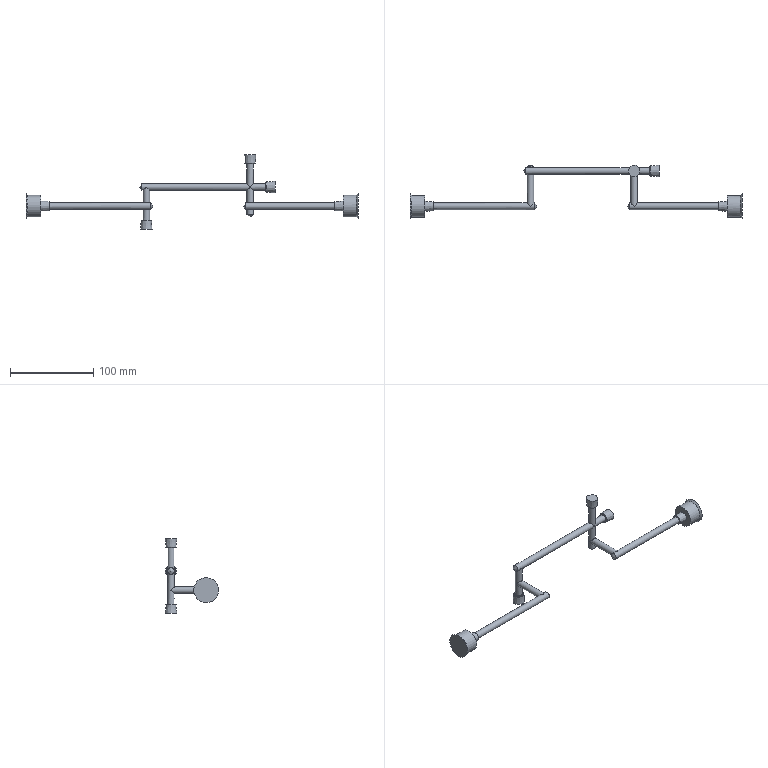Part | STEP file | COOLING-COR_id198_x_t | 1 solid | 37 faces | box 400 x 64.384 x 90 mm | volume 53366 mm3 | cone 14 | plane 12 | cylinder 11 | commonest cylinder face diameters 8 x9 26 x2
STEP:
#1=CARTESIAN_POINT('',(-200.,-80.5,0.));
#2=VERTEX_POINT('',#1);
#3=CARTESIAN_POINT('',(-200.,-80.5,-15.));
#4=DIRECTION('',(1.,0.,0.));
#5=DIRECTION('',(0.,0.,1.));
#6=AXIS2_PLACEMENT_3D('',#3,#4,#5);
#7=CIRCLE('',#6,15.);
#8=EDGE_CURVE('',#2,#2,#7,.T.);
#9=ORIENTED_EDGE('',*,*,#8,.F.);
#10=EDGE_LOOP('',(#9));
#11=FACE_OUTER_BOUND('',#10,.T.);
#12=CARTESIAN_POINT('',(-200.,-80.5,-15.));
#13=DIRECTION('',(1.,0.,0.));
#14=DIRECTION('',(0.,0.,-1.));
#15=AXIS2_PLACEMENT_3D('',#12,#13,#14);
#16=PLANE('',#15);
#17=ADVANCED_FACE('',(#11),#16,.F.);
#18=CARTESIAN_POINT('',(200.,-65.5,-15.));
#19=VERTEX_POINT('',#18);
#20=CARTESIAN_POINT('',(200.,-80.5,-15.));
#21=DIRECTION('',(-1.,0.,0.));
#22=DIRECTION('',(0.,1.,0.));
#23=AXIS2_PLACEMENT_3D('',#20,#21,#22);
#24=CIRCLE('',#23,15.);
#25=EDGE_CURVE('',#19,#19,#24,.T.);
#26=ORIENTED_EDGE('',*,*,#25,.F.);
#27=EDGE_LOOP('',(#26));
#28=FACE_OUTER_BOUND('',#27,.T.);
#29=CARTESIAN_POINT('',(200.,-80.5,-15.));
#30=DIRECTION('',(1.,0.,0.));
#31=DIRECTION('',(0.,0.,-1.));
#32=AXIS2_PLACEMENT_3D('',#29,#30,#31);
#33=PLANE('',#32);
#34=ADVANCED_FACE('',(#28),#33,.T.);
#35=ORIENTED_EDGE('',*,*,#8,.T.);
#36=EDGE_LOOP('',(#35));
#37=FACE_BOUND('',#36,.T.);
#38=CARTESIAN_POINT('',(-198.,-80.5,-28.));
#39=VERTEX_POINT('',#38);
#40=CARTESIAN_POINT('',(-198.,-80.5,-15.));
#41=DIRECTION('',(1.,0.,0.));
#42=DIRECTION('',(0.,0.,-1.));
#43=AXIS2_PLACEMENT_3D('',#40,#41,#42);
#44=CIRCLE('',#43,13.);
#45=EDGE_CURVE('',#39,#39,#44,.T.);
#46=ORIENTED_EDGE('',*,*,#45,.F.);
#47=EDGE_LOOP('',(#46));
#48=FACE_BOUND('',#47,.T.);
#49=CARTESIAN_POINT('',(-200.,-80.5,-15.));
#50=DIRECTION('',(-1.,0.,0.));
#51=DIRECTION('',(0.,0.,1.));
#52=AXIS2_PLACEMENT_3D('',#49,#50,#51);
#53=CONICAL_SURFACE('',#52,15.,45.);
#54=ADVANCED_FACE('',(#37,#48),#53,.T.);
#55=CARTESIAN_POINT('',(198.,-80.5,-28.));
#56=VERTEX_POINT('',#55);
#57=CARTESIAN_POINT('',(198.,-80.5,-15.));
#58=DIRECTION('',(-1.,0.,0.));
#59=DIRECTION('',(0.,0.,-1.));
#60=AXIS2_PLACEMENT_3D('',#57,#58,#59);
#61=CIRCLE('',#60,13.);
#62=EDGE_CURVE('',#56,#56,#61,.T.);
#63=ORIENTED_EDGE('',*,*,#62,.F.);
#64=EDGE_LOOP('',(#63));
#65=FACE_BOUND('',#64,.T.);
#66=ORIENTED_EDGE('',*,*,#25,.T.);
#67=EDGE_LOOP('',(#66));
#68=FACE_BOUND('',#67,.T.);
#69=CARTESIAN_POINT('',(200.,-80.5,-15.));
#70=DIRECTION('',(1.,0.,0.));
#71=DIRECTION('',(0.,1.,0.));
#72=AXIS2_PLACEMENT_3D('',#69,#70,#71);
#73=CONICAL_SURFACE('',#72,15.,45.);
#74=ADVANCED_FACE('',(#65,#68),#73,.T.);
#75=ORIENTED_EDGE('',*,*,#45,.T.);
#76=EDGE_LOOP('',(#75));
#77=FACE_BOUND('',#76,.T.);
#78=CARTESIAN_POINT('',(-182.001,-80.5,-28.));
#79=VERTEX_POINT('',#78);
#80=CARTESIAN_POINT('',(-182.001,-80.5,-15.));
#81=DIRECTION('',(1.,0.,0.));
#82=DIRECTION('',(0.,0.,-1.));
#83=AXIS2_PLACEMENT_3D('',#80,#81,#82);
#84=CIRCLE('',#83,13.);
#85=EDGE_CURVE('',#79,#79,#84,.T.);
#86=ORIENTED_EDGE('',*,*,#85,.F.);
#87=EDGE_LOOP('',(#86));
#88=FACE_BOUND('',#87,.T.);
#89=CARTESIAN_POINT('',(-207.638,-80.5,-15.));
#90=DIRECTION('',(1.,0.,0.));
#91=DIRECTION('',(0.,0.,-1.));
#92=AXIS2_PLACEMENT_3D('',#89,#90,#91);
#93=CYLINDRICAL_SURFACE('',#92,13.);
#94=ADVANCED_FACE('',(#77,#88),#93,.T.);
#95=CARTESIAN_POINT('',(182.001,-80.5,-28.));
#96=VERTEX_POINT('',#95);
#97=CARTESIAN_POINT('',(182.001,-80.5,-15.));
#98=DIRECTION('',(1.,0.,0.));
#99=DIRECTION('',(0.,0.,-1.));
#100=AXIS2_PLACEMENT_3D('',#97,#98,#99);
#101=CIRCLE('',#100,13.);
#102=EDGE_CURVE('',#96,#96,#101,.T.);
#103=ORIENTED_EDGE('',*,*,#102,.T.);
#104=EDGE_LOOP('',(#103));
#105=FACE_BOUND('',#104,.T.);
#106=ORIENTED_EDGE('',*,*,#62,.T.);
#107=EDGE_LOOP('',(#106));
#108=FACE_BOUND('',#107,.T.);
#109=CARTESIAN_POINT('',(55.348,-80.5,-15.));
#110=DIRECTION('',(1.,0.,0.));
#111=DIRECTION('',(0.,0.,-1.));
#112=AXIS2_PLACEMENT_3D('',#109,#110,#111);
#113=CYLINDRICAL_SURFACE('',#112,13.);
#114=ADVANCED_FACE('',(#105,#108),#113,.T.);
#115=CARTESIAN_POINT('',(-182.001,-80.5,-9.045));
#116=VERTEX_POINT('',#115);
#117=CARTESIAN_POINT('',(-182.001,-80.5,-15.));
#118=DIRECTION('',(1.,0.,0.));
#119=DIRECTION('',(0.,0.,1.));
#120=AXIS2_PLACEMENT_3D('',#117,#118,#119);
#121=CIRCLE('',#120,5.955);
#122=EDGE_CURVE('',#116,#116,#121,.T.);
#123=ORIENTED_EDGE('',*,*,#122,.F.);
#124=EDGE_LOOP('',(#123));
#125=FACE_BOUND('',#124,.T.);
#126=ORIENTED_EDGE('',*,*,#85,.T.);
#127=EDGE_LOOP('',(#126));
#128=FACE_BOUND('',#127,.T.);
#129=CARTESIAN_POINT('',(-182.001,-80.5,-15.));
#130=DIRECTION('',(1.,0.,0.));
#131=DIRECTION('',(0.,0.,-1.));
#132=AXIS2_PLACEMENT_3D('',#129,#130,#131);
#133=PLANE('',#132);
#134=ADVANCED_FACE('',(#125,#128),#133,.T.);
#135=CARTESIAN_POINT('',(-61.884,-38.,-43.));
#136=VERTEX_POINT('',#135);
#137=CARTESIAN_POINT('',(-55.,-38.,-43.));
#138=DIRECTION('',(0.,0.,1.));
#139=DIRECTION('',(-1.,0.,0.));
#140=AXIS2_PLACEMENT_3D('',#137,#138,#139);
#141=CIRCLE('',#140,6.884);
#142=EDGE_CURVE('',#136,#136,#141,.T.);
#143=ORIENTED_EDGE('',*,*,#142,.F.);
#144=EDGE_LOOP('',(#143));
#145=FACE_OUTER_BOUND('',#144,.T.);
#146=CARTESIAN_POINT('',(-55.,-38.,-43.));
#147=DIRECTION('',(0.,0.,-1.));
#148=DIRECTION('',(-1.,0.,0.));
#149=AXIS2_PLACEMENT_3D('',#146,#147,#148);
#150=PLANE('',#149);
#151=ADVANCED_FACE('',(#145),#150,.T.);
#152=CARTESIAN_POINT('',(182.001,-80.5,-20.955));
#153=VERTEX_POINT('',#152);
#154=CARTESIAN_POINT('',(182.001,-80.5,-15.));
#155=DIRECTION('',(-1.,0.,0.));
#156=DIRECTION('',(0.,0.,-1.));
#157=AXIS2_PLACEMENT_3D('',#154,#155,#156);
#158=CIRCLE('',#157,5.955);
#159=EDGE_CURVE('',#153,#153,#158,.T.);
#160=ORIENTED_EDGE('',*,*,#159,.F.);
#161=EDGE_LOOP('',(#160));
#162=FACE_BOUND('',#161,.T.);
#163=ORIENTED_EDGE('',*,*,#102,.F.);
#164=EDGE_LOOP('',(#163));
#165=FACE_BOUND('',#164,.T.);
#166=CARTESIAN_POINT('',(182.001,-80.5,-15.));
#167=DIRECTION('',(1.,0.,0.));
#168=DIRECTION('',(0.,0.,-1.));
#169=AXIS2_PLACEMENT_3D('',#166,#167,#168);
#170=PLANE('',#169);
#171=ADVANCED_FACE('',(#162,#165),#170,.F.);
#172=CARTESIAN_POINT('',(100.,-38.,1.116));
#173=VERTEX_POINT('',#172);
#174=CARTESIAN_POINT('',(100.,-38.,8.));
#175=DIRECTION('',(-1.,0.,0.));
#176=DIRECTION('',(0.,0.,-1.));
#177=AXIS2_PLACEMENT_3D('',#174,#175,#176);
#178=CIRCLE('',#177,6.884);
#179=EDGE_CURVE('',#173,#173,#178,.T.);
#180=ORIENTED_EDGE('',*,*,#179,.F.);
#181=EDGE_LOOP('',(#180));
#182=FACE_OUTER_BOUND('',#181,.T.);
#183=CARTESIAN_POINT('',(100.,-38.,8.));
#184=DIRECTION('',(-1.,0.,0.));
#185=DIRECTION('',(0.,0.,1.));
#186=AXIS2_PLACEMENT_3D('',#183,#184,#185);
#187=PLANE('',#186);
#188=ADVANCED_FACE('',(#182),#187,.F.);
#189=CARTESIAN_POINT('',(76.884,-38.,47.));
#190=VERTEX_POINT('',#189);
#191=CARTESIAN_POINT('',(70.,-38.,47.));
#192=DIRECTION('',(0.,0.,-1.));
#193=DIRECTION('',(1.,0.,0.));
#194=AXIS2_PLACEMENT_3D('',#191,#192,#193);
#195=CIRCLE('',#194,6.884);
#196=EDGE_CURVE('',#190,#190,#195,.T.);
#197=ORIENTED_EDGE('',*,*,#196,.F.);
#198=EDGE_LOOP('',(#197));
#199=FACE_OUTER_BOUND('',#198,.T.);
#200=CARTESIAN_POINT('',(70.,-38.,47.));
#201=DIRECTION('',(0.,0.,1.));
#202=DIRECTION('',(1.,0.,0.));
#203=AXIS2_PLACEMENT_3D('',#200,#201,#202);
#204=PLANE('',#203);
#205=ADVANCED_FACE('',(#199),#204,.T.);
#206=ORIENTED_EDGE('',*,*,#122,.T.);
#207=EDGE_LOOP('',(#206));
#208=FACE_BOUND('',#207,.T.);
#209=CARTESIAN_POINT('',(-172.001,-80.5,-9.5));
#210=VERTEX_POINT('',#209);
#211=CARTESIAN_POINT('',(-172.001,-80.5,-15.));
#212=DIRECTION('',(1.,0.,0.));
#213=DIRECTION('',(0.,0.,1.));
#214=AXIS2_PLACEMENT_3D('',#211,#212,#213);
#215=CIRCLE('',#214,5.5);
#216=EDGE_CURVE('',#210,#210,#215,.T.);
#217=ORIENTED_EDGE('',*,*,#216,.F.);
#218=EDGE_LOOP('',(#217));
#219=FACE_BOUND('',#218,.T.);
#220=CARTESIAN_POINT('',(-182.001,-80.5,-15.));
#221=DIRECTION('',(-1.,0.,0.));
#222=DIRECTION('',(0.,0.,1.));
#223=AXIS2_PLACEMENT_3D('',#220,#221,#222);
#224=CONICAL_SURFACE('',#223,5.955,2.603);
#225=ADVANCED_FACE('',(#208,#219),#224,.T.);
#226=ORIENTED_EDGE('',*,*,#142,.T.);
#227=EDGE_LOOP('',(#226));
#228=FACE_BOUND('',#227,.T.);
#229=CARTESIAN_POINT('',(-48.758,-38.,-32.5));
#230=VERTEX_POINT('',#229);
#231=CARTESIAN_POINT('',(-55.,-38.,-32.5));
#232=DIRECTION('',(0.,0.,1.));
#233=DIRECTION('',(1.,0.,0.));
#234=AXIS2_PLACEMENT_3D('',#231,#232,#233);
#235=CIRCLE('',#234,6.242);
#236=EDGE_CURVE('',#230,#230,#235,.T.);
#237=ORIENTED_EDGE('',*,*,#236,.F.);
#238=EDGE_LOOP('',(#237));
#239=FACE_BOUND('',#238,.T.);
#240=CARTESIAN_POINT('',(-55.,-38.,-43.));
#241=DIRECTION('',(0.,0.,-1.));
#242=DIRECTION('',(-1.,0.,0.));
#243=AXIS2_PLACEMENT_3D('',#240,#241,#242);
#244=CONICAL_SURFACE('',#243,6.884,3.5);
#245=ADVANCED_FACE('',(#228,#239),#244,.T.);
#246=CARTESIAN_POINT('',(172.001,-80.5,-20.5));
#247=VERTEX_POINT('',#246);
#248=CARTESIAN_POINT('',(172.001,-80.5,-15.));
#249=DIRECTION('',(1.,0.,0.));
#250=DIRECTION('',(0.,0.,-1.));
#251=AXIS2_PLACEMENT_3D('',#248,#249,#250);
#252=CIRCLE('',#251,5.5);
#253=EDGE_CURVE('',#247,#247,#252,.T.);
#254=ORIENTED_EDGE('',*,*,#253,.T.);
#255=EDGE_LOOP('',(#254));
#256=FACE_BOUND('',#255,.T.);
#257=ORIENTED_EDGE('',*,*,#159,.T.);
#258=EDGE_LOOP('',(#257));
#259=FACE_BOUND('',#258,.T.);
#260=CARTESIAN_POINT('',(182.001,-80.5,-15.));
#261=DIRECTION('',(1.,0.,0.));
#262=DIRECTION('',(0.,0.,-1.));
#263=AXIS2_PLACEMENT_3D('',#260,#261,#262);
#264=CONICAL_SURFACE('',#263,5.955,2.603);
#265=ADVANCED_FACE('',(#256,#259),#264,.T.);
#266=ORIENTED_EDGE('',*,*,#179,.T.);
#267=EDGE_LOOP('',(#266));
#268=FACE_BOUND('',#267,.T.);
#269=CARTESIAN_POINT('',(89.5,-38.,14.242));
#270=VERTEX_POINT('',#269);
#271=CARTESIAN_POINT('',(89.5,-38.,8.));
#272=DIRECTION('',(-1.,0.,0.));
#273=DIRECTION('',(0.,0.,1.));
#274=AXIS2_PLACEMENT_3D('',#271,#272,#273);
#275=CIRCLE('',#274,6.242);
#276=EDGE_CURVE('',#270,#270,#275,.T.);
#277=ORIENTED_EDGE('',*,*,#276,.F.);
#278=EDGE_LOOP('',(#277));
#279=FACE_BOUND('',#278,.T.);
#280=CARTESIAN_POINT('',(100.,-38.,8.));
#281=DIRECTION('',(1.,0.,0.));
#282=DIRECTION('',(0.,0.,-1.));
#283=AXIS2_PLACEMENT_3D('',#280,#281,#282);
#284=CONICAL_SURFACE('',#283,6.884,3.5);
#285=ADVANCED_FACE('',(#268,#279),#284,.T.);
#286=CARTESIAN_POINT('',(63.758,-38.,36.503));
#287=VERTEX_POINT('',#286);
#288=CARTESIAN_POINT('',(70.,-38.,36.503));
#289=DIRECTION('',(0.,0.,-1.));
#290=DIRECTION('',(-1.,0.,0.));
#291=AXIS2_PLACEMENT_3D('',#288,#289,#290);
#292=CIRCLE('',#291,6.242);
#293=EDGE_CURVE('',#287,#287,#292,.T.);
#294=ORIENTED_EDGE('',*,*,#293,.F.);
#295=EDGE_LOOP('',(#294));
#296=FACE_BOUND('',#295,.T.);
#297=ORIENTED_EDGE('',*,*,#196,.T.);
#298=EDGE_LOOP('',(#297));
#299=FACE_BOUND('',#298,.T.);
#300=CARTESIAN_POINT('',(70.,-38.,47.));
#301=DIRECTION('',(0.,0.,1.));
#302=DIRECTION('',(1.,0.,0.));
#303=AXIS2_PLACEMENT_3D('',#300,#301,#302);
#304=CONICAL_SURFACE('',#303,6.884,3.5);
#305=ADVANCED_FACE('',(#296,#299),#304,.T.);
#306=CARTESIAN_POINT('',(-172.001,-80.5,-19.));
#307=VERTEX_POINT('',#306);
#308=CARTESIAN_POINT('',(-172.001,-80.5,-15.));
#309=DIRECTION('',(1.,0.,0.));
#310=DIRECTION('',(0.,0.,-1.));
#311=AXIS2_PLACEMENT_3D('',#308,#309,#310);
#312=CIRCLE('',#311,4.);
#313=EDGE_CURVE('',#307,#307,#312,.T.);
#314=ORIENTED_EDGE('',*,*,#313,.F.);
#315=EDGE_LOOP('',(#314));
#316=FACE_BOUND('',#315,.T.);
#317=ORIENTED_EDGE('',*,*,#216,.T.);
#318=EDGE_LOOP('',(#317));
#319=FACE_BOUND('',#318,.T.);
#320=CARTESIAN_POINT('',(-172.001,-80.5,-15.));
#321=DIRECTION('',(1.,0.,0.));
#322=DIRECTION('',(0.,0.,-1.));
#323=AXIS2_PLACEMENT_3D('',#320,#321,#322);
#324=PLANE('',#323);
#325=ADVANCED_FACE('',(#316,#319),#324,.T.);
#326=CARTESIAN_POINT('',(-47.236,-80.5,-15.));
#327=VERTEX_POINT('',#326);
#328=VERTEX_LOOP('',#327);
#329=FACE_BOUND('',#328,.T.);
#330=CARTESIAN_POINT('',(-49.459,-80.5,-19.));
#331=VERTEX_POINT('',#330);
#332=CARTESIAN_POINT('',(-49.459,-80.5,-15.));
#333=DIRECTION('',(-1.,0.,0.));
#334=DIRECTION('',(0.,0.,-1.));
#335=AXIS2_PLACEMENT_3D('',#332,#333,#334);
#336=CIRCLE('',#335,4.);
#337=EDGE_CURVE('',#331,#331,#336,.T.);
#338=ORIENTED_EDGE('',*,*,#337,.F.);
#339=EDGE_LOOP('',(#338));
#340=FACE_BOUND('',#339,.T.);
#341=CARTESIAN_POINT('',(-49.459,-80.5,-15.));
#342=DIRECTION('',(-1.,0.,0.));
#343=DIRECTION('',(0.,-1.,0.));
#344=AXIS2_PLACEMENT_3D('',#341,#342,#343);
#345=CONICAL_SURFACE('',#344,4.,60.942);
#346=ADVANCED_FACE('',(#329,#340),#345,.T.);
#347=ORIENTED_EDGE('',*,*,#236,.T.);
#348=EDGE_LOOP('',(#347));
#349=FACE_BOUND('',#348,.T.);
#350=CARTESIAN_POINT('',(-60.742,-38.,-32.));
#351=VERTEX_POINT('',#350);
#352=CARTESIAN_POINT('',(-55.,-38.,-32.));
#353=DIRECTION('',(0.,0.,-1.));
#354=DIRECTION('',(-1.,0.,0.));
#355=AXIS2_PLACEMENT_3D('',#352,#353,#354);
#356=CIRCLE('',#355,5.742);
#357=EDGE_CURVE('',#351,#351,#356,.T.);
#358=ORIENTED_EDGE('',*,*,#357,.T.);
#359=EDGE_LOOP('',(#358));
#360=FACE_BOUND('',#359,.T.);
#361=CARTESIAN_POINT('',(-55.,-38.,-32.5));
#362=DIRECTION('',(0.,0.,-1.));
#363=DIRECTION('',(-1.,0.,0.));
#364=AXIS2_PLACEMENT_3D('',#361,#362,#363);
#365=CONICAL_SURFACE('',#364,6.242,45.);
#366=ADVANCED_FACE('',(#349,#360),#365,.T.);
#367=CARTESIAN_POINT('',(172.001,-80.5,-19.));
#368=VERTEX_POINT('',#367);
#369=CARTESIAN_POINT('',(172.001,-80.5,-15.));
#370=DIRECTION('',(-1.,0.,0.));
#371=DIRECTION('',(0.,0.,-1.));
#372=AXIS2_PLACEMENT_3D('',#369,#370,#371);
#373=CIRCLE('',#372,4.);
#374=EDGE_CURVE('',#368,#368,#373,.T.);
#375=ORIENTED_EDGE('',*,*,#374,.F.);
#376=EDGE_LOOP('',(#375));
#377=FACE_BOUND('',#376,.T.);
#378=ORIENTED_EDGE('',*,*,#253,.F.);
#379=EDGE_LOOP('',(#378));
#380=FACE_BOUND('',#379,.T.);
#381=CARTESIAN_POINT('',(172.001,-80.5,-15.));
#382=DIRECTION('',(1.,0.,0.));
#383=DIRECTION('',(0.,0.,-1.));
#384=AXIS2_PLACEMENT_3D('',#381,#382,#383);
#385=PLANE('',#384);
#386=ADVANCED_FACE('',(#377,#380),#385,.F.);
#387=CARTESIAN_POINT('',(64.459,-80.5,-19.));
#388=VERTEX_POINT('',#387);
#389=CARTESIAN_POINT('',(64.459,-80.5,-15.));
#390=DIRECTION('',(1.,0.,0.));
#391=DIRECTION('',(0.,0.,-1.));
#392=AXIS2_PLACEMENT_3D('',#389,#390,#391);
#393=CIRCLE('',#392,4.);
#394=EDGE_CURVE('',#388,#388,#393,.T.);
#395=ORIENTED_EDGE('',*,*,#394,.F.);
#396=EDGE_LOOP('',(#395));
#397=FACE_BOUND('',#396,.T.);
#398=CARTESIAN_POINT('',(62.236,-80.5,-15.));
#399=VERTEX_POINT('',#398);
#400=VERTEX_LOOP('',#399);
#401=FACE_BOUND('',#400,.T.);
#402=CARTESIAN_POINT('',(64.459,-80.5,-15.));
#403=DIRECTION('',(1.,0.,0.));
#404=DIRECTION('',(0.,0.,-1.));
#405=AXIS2_PLACEMENT_3D('',#402,#403,#404);
#406=CONICAL_SURFACE('',#405,4.,60.942);
#407=ADVANCED_FACE('',(#397,#401),#406,.T.);
#408=ORIENTED_EDGE('',*,*,#276,.T.);
#409=EDGE_LOOP('',(#408));
#410=FACE_BOUND('',#409,.T.);
#411=CARTESIAN_POINT('',(89.,-38.,2.258));
#412=VERTEX_POINT('',#411);
#413=CARTESIAN_POINT('',(89.,-38.,8.));
#414=DIRECTION('',(-1.,0.,0.));
#415=DIRECTION('',(0.,0.,-1.));
#416=AXIS2_PLACEMENT_3D('',#413,#414,#415);
#417=CIRCLE('',#416,5.742);
#418=EDGE_CURVE('',#412,#412,#417,.T.);
#419=ORIENTED_EDGE('',*,*,#418,.F.);
#420=EDGE_LOOP('',(#419));
#421=FACE_BOUND('',#420,.T.);
#422=CARTESIAN_POINT('',(89.5,-38.,8.));
#423=DIRECTION('',(1.,0.,0.));
#424=DIRECTION('',(0.,0.,-1.));
#425=AXIS2_PLACEMENT_3D('',#422,#423,#424);
#426=CONICAL_SURFACE('',#425,6.242,45.);
#427=ADVANCED_FACE('',(#410,#421),#426,.T.);
#428=CARTESIAN_POINT('',(75.742,-38.,36.003));
#429=VERTEX_POINT('',#428);
#430=CARTESIAN_POINT('',(70.,-38.,36.003));
#431=DIRECTION('',(0.,0.,1.));
#432=DIRECTION('',(1.,0.,0.));
#433=AXIS2_PLACEMENT_3D('',#430,#431,#432);
#434=CIRCLE('',#433,5.742);
#435=EDGE_CURVE('',#429,#429,#434,.T.);
#436=ORIENTED_EDGE('',*,*,#435,.T.);
#437=EDGE_LOOP('',(#436));
#438=FACE_BOUND('',#437,.T.);
#439=ORIENTED_EDGE('',*,*,#293,.T.);
#440=EDGE_LOOP('',(#439));
#441=FACE_BOUND('',#440,.T.);
#442=CARTESIAN_POINT('',(70.,-38.,36.503));
#443=DIRECTION('',(0.,0.,1.));
#444=DIRECTION('',(1.,0.,0.));
#445=AXIS2_PLACEMENT_3D('',#442,#443,#444);
#446=CONICAL_SURFACE('',#445,6.242,45.);
#447=ADVANCED_FACE('',(#438,#441),#446,.T.);
#448=ORIENTED_EDGE('',*,*,#313,.T.);
#449=EDGE_LOOP('',(#448));
#450=FACE_BOUND('',#449,.T.);
#451=ORIENTED_EDGE('',*,*,#337,.T.);
#452=EDGE_LOOP('',(#451));
#453=FACE_BOUND('',#452,.T.);
#454=CARTESIAN_POINT('',(-55.,-80.5,-19.));
#455=VERTEX_POINT('',#454);
#456=CARTESIAN_POINT('',(-55.,-80.5,-11.));
#457=VERTEX_POINT('',#456);
#458=CARTESIAN_POINT('',(-55.,-80.5,-15.));
#459=DIRECTION('',(0.7071,0.7071,0.));
#460=DIRECTION('',(0.7071,-0.7071,0.));
#461=AXIS2_PLACEMENT_3D('',#458,#459,#460);
#462=ELLIPSE('',#461,5.657,4.);
#463=EDGE_CURVE('',#455,#457,#462,.T.);
#464=ORIENTED_EDGE('',*,*,#463,.F.);
#465=CARTESIAN_POINT('',(-55.,-80.5,-15.));
#466=DIRECTION('',(-0.7071,0.7071,0.));
#467=DIRECTION('',(0.7071,0.7071,0.));
#468=AXIS2_PLACEMENT_3D('',#465,#466,#467);
#469=ELLIPSE('',#468,5.657,4.);
#470=EDGE_CURVE('',#457,#455,#469,.T.);
#471=ORIENTED_EDGE('',*,*,#470,.F.);
#472=EDGE_LOOP('',(#464,#471));
#473=FACE_BOUND('',#472,.T.);
#474=CARTESIAN_POINT('',(-207.638,-80.5,-15.));
#475=DIRECTION('',(1.,0.,0.));
#476=DIRECTION('',(0.,0.,-1.));
#477=AXIS2_PLACEMENT_3D('',#474,#475,#476);
#478=CYLINDRICAL_SURFACE('',#477,4.);
#479=ADVANCED_FACE('',(#450,#453,#473),#478,.T.);
#480=CARTESIAN_POINT('',(-59.,-38.,-32.));
#481=VERTEX_POINT('',#480);
#482=CARTESIAN_POINT('',(-55.,-38.,-32.));
#483=DIRECTION('',(0.,0.,1.));
#484=DIRECTION('',(-1.,0.,0.));
#485=AXIS2_PLACEMENT_3D('',#482,#483,#484);
#486=CIRCLE('',#485,4.);
#487=EDGE_CURVE('',#481,#481,#486,.T.);
#488=ORIENTED_EDGE('',*,*,#487,.F.);
#489=EDGE_LOOP('',(#488));
#490=FACE_BOUND('',#489,.T.);
#491=ORIENTED_EDGE('',*,*,#357,.F.);
#492=EDGE_LOOP('',(#491));
#493=FACE_BOUND('',#492,.T.);
#494=CARTESIAN_POINT('',(-55.,-38.,-32.));
#495=DIRECTION('',(0.,0.,-1.));
#496=DIRECTION('',(-1.,0.,0.));
#497=AXIS2_PLACEMENT_3D('',#494,#495,#496);
#498=PLANE('',#497);
#499=ADVANCED_FACE('',(#490,#493),#498,.F.);
#500=ORIENTED_EDGE('',*,*,#374,.T.);
#501=EDGE_LOOP('',(#500));
#502=FACE_BOUND('',#501,.T.);
#503=ORIENTED_EDGE('',*,*,#394,.T.);
#504=EDGE_LOOP('',(#503));
#505=FACE_BOUND('',#504,.T.);
#506=CARTESIAN_POINT('',(70.,-80.5,-19.));
#507=VERTEX_POINT('',#506);
#508=CARTESIAN_POINT('',(70.,-80.5,-11.));
#509=VERTEX_POINT('',#508);
#510=CARTESIAN_POINT('',(70.,-80.5,-15.));
#511=DIRECTION('',(0.7071,0.7071,0.));
#512=DIRECTION('',(0.7071,-0.7071,0.));
#513=AXIS2_PLACEMENT_3D('',#510,#511,#512);
#514=ELLIPSE('',#513,5.657,4.);
#515=EDGE_CURVE('',#507,#509,#514,.T.);
#516=ORIENTED_EDGE('',*,*,#515,.F.);
#517=CARTESIAN_POINT('',(70.,-80.5,-15.));
#518=DIRECTION('',(-0.7071,0.7071,0.));
#519=DIRECTION('',(0.7071,0.7071,0.));
#520=AXIS2_PLACEMENT_3D('',#517,#518,#519);
#521=ELLIPSE('',#520,5.657,4.);
#522=EDGE_CURVE('',#509,#507,#521,.T.);
#523=ORIENTED_EDGE('',*,*,#522,.F.);
#524=EDGE_LOOP('',(#516,#523));
#525=FACE_BOUND('',#524,.T.);
#526=CARTESIAN_POINT('',(55.348,-80.5,-15.));
#527=DIRECTION('',(1.,0.,0.));
#528=DIRECTION('',(0.,0.,-1.));
#529=AXIS2_PLACEMENT_3D('',#526,#527,#528);
#530=CYLINDRICAL_SURFACE('',#529,4.);
#531=ADVANCED_FACE('',(#502,#505,#525),#530,.T.);
#532=CARTESIAN_POINT('',(70.,-38.,-27.764));
#533=VERTEX_POINT('',#532);
#534=VERTEX_LOOP('',#533);
#535=FACE_BOUND('',#534,.T.);
#536=CARTESIAN_POINT('',(74.,-38.,-25.541));
#537=VERTEX_POINT('',#536);
#538=CARTESIAN_POINT('',(70.,-38.,-25.541));
#539=DIRECTION('',(0.,0.,1.));
#540=DIRECTION('',(1.,0.,0.));
#541=AXIS2_PLACEMENT_3D('',#538,#539,#540);
#542=CIRCLE('',#541,4.);
#543=EDGE_CURVE('',#537,#537,#542,.T.);
#544=ORIENTED_EDGE('',*,*,#543,.F.);
#545=EDGE_LOOP('',(#544));
#546=FACE_BOUND('',#545,.T.);
#547=CARTESIAN_POINT('',(70.,-38.,-25.541));
#548=DIRECTION('',(0.,0.,1.));
#549=DIRECTION('',(1.,0.,0.));
#550=AXIS2_PLACEMENT_3D('',#547,#548,#549);
#551=CONICAL_SURFACE('',#550,4.,60.942);
#552=ADVANCED_FACE('',(#535,#546),#551,.T.);
#553=CARTESIAN_POINT('',(89.,-38.,12.));
#554=VERTEX_POINT('',#553);
#555=CARTESIAN_POINT('',(89.,-38.,8.));
#556=DIRECTION('',(-1.,0.,0.));
#557=DIRECTION('',(0.,0.,1.));
#558=AXIS2_PLACEMENT_3D('',#555,#556,#557);
#559=CIRCLE('',#558,4.);
#560=EDGE_CURVE('',#554,#554,#559,.T.);
#561=ORIENTED_EDGE('',*,*,#560,.F.);
#562=EDGE_LOOP('',(#561));
#563=FACE_BOUND('',#562,.T.);
#564=ORIENTED_EDGE('',*,*,#418,.T.);
#565=EDGE_LOOP('',(#564));
#566=FACE_BOUND('',#565,.T.);
#567=CARTESIAN_POINT('',(89.,-38.,8.));
#568=DIRECTION('',(-1.,0.,0.));
#569=DIRECTION('',(0.,0.,1.));
#570=AXIS2_PLACEMENT_3D('',#567,#568,#569);
#571=PLANE('',#570);
#572=ADVANCED_FACE('',(#563,#566),#571,.T.);
#573=CARTESIAN_POINT('',(74.,-38.,36.003));
#574=VERTEX_POINT('',#573);
#575=CARTESIAN_POINT('',(70.,-38.,36.003));
#576=DIRECTION('',(0.,0.,-1.));
#577=DIRECTION('',(1.,0.,0.));
#578=AXIS2_PLACEMENT_3D('',#575,#576,#577);
#579=CIRCLE('',#578,4.);
#580=EDGE_CURVE('',#574,#574,#579,.T.);
#581=ORIENTED_EDGE('',*,*,#580,.F.);
#582=EDGE_LOOP('',(#581));
#583=FACE_BOUND('',#582,.T.);
#584=ORIENTED_EDGE('',*,*,#435,.F.);
#585=EDGE_LOOP('',(#584));
#586=FACE_BOUND('',#585,.T.);
#587=CARTESIAN_POINT('',(70.,-38.,36.003));
#588=DIRECTION('',(0.,0.,1.));
#589=DIRECTION('',(1.,0.,0.));
#590=AXIS2_PLACEMENT_3D('',#587,#588,#589);
#591=PLANE('',#590);
#592=ADVANCED_FACE('',(#583,#586),#591,.F.);
#593=ORIENTED_EDGE('',*,*,#470,.T.);
#594=ORIENTED_EDGE('',*,*,#463,.T.);
#595=EDGE_LOOP('',(#593,#594));
#596=FACE_BOUND('',#595,.T.);
#597=CARTESIAN_POINT('',(-59.,-38.,-15.));
#598=VERTEX_POINT('',#597);
#599=CARTESIAN_POINT('',(-51.,-38.,-15.));
#600=VERTEX_POINT('',#599);
#601=CARTESIAN_POINT('',(-55.,-38.,-15.));
#602=DIRECTION('',(0.,0.7071,0.7071));
#603=DIRECTION('',(0.,0.7071,-0.7071));
#604=AXIS2_PLACEMENT_3D('',#601,#602,#603);
#605=ELLIPSE('',#604,5.657,4.);
#606=EDGE_CURVE('',#598,#600,#605,.T.);
#607=ORIENTED_EDGE('',*,*,#606,.F.);
#608=CARTESIAN_POINT('',(-55.,-38.,-15.));
#609=DIRECTION('',(0.,0.7071,-0.7071));
#610=DIRECTION('',(0.,-0.7071,-0.7071));
#611=AXIS2_PLACEMENT_3D('',#608,#609,#610);
#612=ELLIPSE('',#611,5.657,4.);
#613=EDGE_CURVE('',#600,#598,#612,.T.);
#614=ORIENTED_EDGE('',*,*,#613,.F.);
#615=EDGE_LOOP('',(#607,#614));
#616=FACE_BOUND('',#615,.T.);
#617=CARTESIAN_POINT('',(-55.,-38.,-15.));
#618=DIRECTION('',(0.,1.,0.));
#619=DIRECTION('',(0.,0.,1.));
#620=AXIS2_PLACEMENT_3D('',#617,#618,#619);
#621=CYLINDRICAL_SURFACE('',#620,4.);
#622=ADVANCED_FACE('',(#596,#616),#621,.T.);
#623=CARTESIAN_POINT('',(74.,-38.,-15.));
#624=VERTEX_POINT('',#623);
#625=CARTESIAN_POINT('',(66.,-38.,-15.));
#626=VERTEX_POINT('',#625);
#627=CARTESIAN_POINT('',(70.,-38.,-15.));
#628=DIRECTION('',(0.,0.7071,-0.7071));
#629=DIRECTION('',(0.,0.7071,0.7071));
#630=AXIS2_PLACEMENT_3D('',#627,#628,#629);
#631=ELLIPSE('',#630,5.657,4.);
#632=EDGE_CURVE('',#624,#626,#631,.T.);
#633=ORIENTED_EDGE('',*,*,#632,.F.);
#634=CARTESIAN_POINT('',(70.,-38.,-15.));
#635=DIRECTION('',(0.,0.7071,0.7071));
#636=DIRECTION('',(0.,-0.7071,0.7071));
#637=AXIS2_PLACEMENT_3D('',#634,#635,#636);
#638=ELLIPSE('',#637,5.657,4.);
#639=EDGE_CURVE('',#626,#624,#638,.T.);
#640=ORIENTED_EDGE('',*,*,#639,.F.);
#641=EDGE_LOOP('',(#633,#640));
#642=FACE_BOUND('',#641,.T.);
#643=ORIENTED_EDGE('',*,*,#522,.T.);
#644=ORIENTED_EDGE('',*,*,#515,.T.);
#645=EDGE_LOOP('',(#643,#644));
#646=FACE_BOUND('',#645,.T.);
#647=CARTESIAN_POINT('',(70.,-38.,-15.));
#648=DIRECTION('',(0.,1.,0.));
#649=DIRECTION('',(0.,0.,1.));
#650=AXIS2_PLACEMENT_3D('',#647,#648,#649);
#651=CYLINDRICAL_SURFACE('',#650,4.);
#652=ADVANCED_FACE('',(#642,#646),#651,.T.);
#653=ORIENTED_EDGE('',*,*,#560,.T.);
#654=EDGE_LOOP('',(#653));
#655=FACE_BOUND('',#654,.T.);
#656=CARTESIAN_POINT('',(70.,-34.,8.));
#657=VERTEX_POINT('',#656);
#658=CARTESIAN_POINT('',(70.,-42.,8.));
#659=VERTEX_POINT('',#658);
#660=CARTESIAN_POINT('',(70.,-38.,8.));
#661=DIRECTION('',(-0.7071,0.,-0.7071));
#662=DIRECTION('',(-0.7071,0.,0.7071));
#663=AXIS2_PLACEMENT_3D('',#660,#661,#662);
#664=ELLIPSE('',#663,5.657,4.);
#665=EDGE_CURVE('',#657,#659,#664,.T.);
#666=ORIENTED_EDGE('',*,*,#665,.F.);
#667=CARTESIAN_POINT('',(70.,-38.,8.));
#668=DIRECTION('',(-0.7071,0.,0.7071));
#669=DIRECTION('',(0.7071,0.,0.7071));
#670=AXIS2_PLACEMENT_3D('',#667,#668,#669);
#671=ELLIPSE('',#670,5.657,4.);
#672=EDGE_CURVE('',#659,#657,#671,.T.);
#673=ORIENTED_EDGE('',*,*,#672,.F.);
#674=EDGE_LOOP('',(#666,#673));
#675=FACE_BOUND('',#674,.T.);
#676=CARTESIAN_POINT('',(108.138,-38.,8.));
#677=DIRECTION('',(-1.,0.,0.));
#678=DIRECTION('',(0.,0.,1.));
#679=AXIS2_PLACEMENT_3D('',#676,#677,#678);
#680=CYLINDRICAL_SURFACE('',#679,4.);
#681=ADVANCED_FACE('',(#655,#675),#680,.T.);
#682=ORIENTED_EDGE('',*,*,#580,.T.);
#683=EDGE_LOOP('',(#682));
#684=FACE_BOUND('',#683,.T.);
#685=ORIENTED_EDGE('',*,*,#672,.T.);
#686=CARTESIAN_POINT('',(70.,-38.,8.));
#687=DIRECTION('',(-0.7071,0.,-0.7071));
#688=DIRECTION('',(-0.7071,0.,0.7071));
#689=AXIS2_PLACEMENT_3D('',#686,#687,#688);
#690=ELLIPSE('',#689,5.657,4.);
#691=EDGE_CURVE('',#659,#657,#690,.T.);
#692=ORIENTED_EDGE('',*,*,#691,.F.);
#693=EDGE_LOOP('',(#685,#692));
#694=FACE_BOUND('',#693,.T.);
#695=CARTESIAN_POINT('',(70.,-38.,-31.502));
#696=DIRECTION('',(0.,0.,1.));
#697=DIRECTION('',(1.,0.,0.));
#698=AXIS2_PLACEMENT_3D('',#695,#696,#697);
#699=CYLINDRICAL_SURFACE('',#698,4.);
#700=ADVANCED_FACE('',(#684,#694),#699,.T.);
#701=CARTESIAN_POINT('',(-62.764,-38.,8.));
#702=VERTEX_POINT('',#701);
#703=VERTEX_LOOP('',#702);
#704=FACE_BOUND('',#703,.T.);
#705=CARTESIAN_POINT('',(-60.541,-38.,12.));
#706=VERTEX_POINT('',#705);
#707=CARTESIAN_POINT('',(-60.541,-38.,8.));
#708=DIRECTION('',(1.,0.,0.));
#709=DIRECTION('',(0.,0.,1.));
#710=AXIS2_PLACEMENT_3D('',#707,#708,#709);
#711=CIRCLE('',#710,4.);
#712=EDGE_CURVE('',#706,#706,#711,.T.);
#713=ORIENTED_EDGE('',*,*,#712,.F.);
#714=EDGE_LOOP('',(#713));
#715=FACE_BOUND('',#714,.T.);
#716=CARTESIAN_POINT('',(-60.541,-38.,8.));
#717=DIRECTION('',(1.,0.,0.));
#718=DIRECTION('',(0.,0.,-1.));
#719=AXIS2_PLACEMENT_3D('',#716,#717,#718);
#720=CONICAL_SURFACE('',#719,4.,60.942);
#721=ADVANCED_FACE('',(#704,#715),#720,.T.);
#722=ORIENTED_EDGE('',*,*,#487,.T.);
#723=EDGE_LOOP('',(#722));
#724=FACE_BOUND('',#723,.T.);
#725=ORIENTED_EDGE('',*,*,#606,.T.);
#726=ORIENTED_EDGE('',*,*,#613,.T.);
#727=EDGE_LOOP('',(#725,#726));
#728=FACE_BOUND('',#727,.T.);
#729=CARTESIAN_POINT('',(-55.,-34.,8.));
#730=VERTEX_POINT('',#729);
#731=CARTESIAN_POINT('',(-55.,-42.,8.));
#732=VERTEX_POINT('',#731);
#733=CARTESIAN_POINT('',(-55.,-38.,8.));
#734=DIRECTION('',(-0.7071,0.,0.7071));
#735=DIRECTION('',(-0.7071,0.,-0.7071));
#736=AXIS2_PLACEMENT_3D('',#733,#734,#735);
#737=ELLIPSE('',#736,5.657,4.);
#738=EDGE_CURVE('',#730,#732,#737,.T.);
#739=ORIENTED_EDGE('',*,*,#738,.F.);
#740=CARTESIAN_POINT('',(-55.,-38.,8.));
#741=DIRECTION('',(0.7071,0.,0.7071));
#742=DIRECTION('',(-0.7071,0.,0.7071));
#743=AXIS2_PLACEMENT_3D('',#740,#741,#742);
#744=ELLIPSE('',#743,5.657,4.);
#745=EDGE_CURVE('',#732,#730,#744,.T.);
#746=ORIENTED_EDGE('',*,*,#745,.F.);
#747=EDGE_LOOP('',(#739,#746));
#748=FACE_BOUND('',#747,.T.);
#749=CARTESIAN_POINT('',(-55.,-38.,10.55));
#750=DIRECTION('',(0.,0.,-1.));
#751=DIRECTION('',(-1.,0.,0.));
#752=AXIS2_PLACEMENT_3D('',#749,#750,#751);
#753=CYLINDRICAL_SURFACE('',#752,4.);
#754=ADVANCED_FACE('',(#724,#728,#748),#753,.T.);
#755=ORIENTED_EDGE('',*,*,#543,.T.);
#756=EDGE_LOOP('',(#755));
#757=FACE_BOUND('',#756,.T.);
#758=ORIENTED_EDGE('',*,*,#639,.T.);
#759=ORIENTED_EDGE('',*,*,#632,.T.);
#760=EDGE_LOOP('',(#758,#759));
#761=FACE_BOUND('',#760,.T.);
#762=CARTESIAN_POINT('',(70.,-38.,8.));
#763=DIRECTION('',(-0.7071,0.,0.7071));
#764=DIRECTION('',(0.7071,0.,0.7071));
#765=AXIS2_PLACEMENT_3D('',#762,#763,#764);
#766=ELLIPSE('',#765,5.657,4.);
#767=EDGE_CURVE('',#657,#659,#766,.T.);
#768=ORIENTED_EDGE('',*,*,#767,.F.);
#769=ORIENTED_EDGE('',*,*,#665,.T.);
#770=EDGE_LOOP('',(#768,#769));
#771=FACE_BOUND('',#770,.T.);
#772=CARTESIAN_POINT('',(70.,-38.,-31.502));
#773=DIRECTION('',(0.,0.,1.));
#774=DIRECTION('',(1.,0.,0.));
#775=AXIS2_PLACEMENT_3D('',#772,#773,#774);
#776=CYLINDRICAL_SURFACE('',#775,4.);
#777=ADVANCED_FACE('',(#757,#761,#771),#776,.T.);
#778=ORIENTED_EDGE('',*,*,#712,.T.);
#779=EDGE_LOOP('',(#778));
#780=FACE_BOUND('',#779,.T.);
#781=ORIENTED_EDGE('',*,*,#745,.T.);
#782=ORIENTED_EDGE('',*,*,#738,.T.);
#783=EDGE_LOOP('',(#781,#782));
#784=FACE_BOUND('',#783,.T.);
#785=ORIENTED_EDGE('',*,*,#691,.T.);
#786=ORIENTED_EDGE('',*,*,#767,.T.);
#787=EDGE_LOOP('',(#785,#786));
#788=FACE_BOUND('',#787,.T.);
#789=CARTESIAN_POINT('',(108.138,-38.,8.));
#790=DIRECTION('',(-1.,0.,0.));
#791=DIRECTION('',(0.,0.,1.));
#792=AXIS2_PLACEMENT_3D('',#789,#790,#791);
#793=CYLINDRICAL_SURFACE('',#792,4.);
#794=ADVANCED_FACE('',(#780,#784,#788),#793,.T.);
#795=CLOSED_SHELL('',(#17,#34,#54,#74,#94,#114,#134,#151,#171,#188,#205,#225,#245,#265,#285,#305,#325,#346,#366,#386,#407,#427,#447,#479,#499,#531,#552,#572,#592,#622,#652,#681,#700,#721,#754,#777,#794));
#796=MANIFOLD_SOLID_BREP('',#795);
#797=(LENGTH_UNIT()NAMED_UNIT(*)SI_UNIT(.MILLI.,.METRE.));
#798=UNCERTAINTY_MEASURE_WITH_UNIT(LENGTH_MEASURE(0.00004123),#797,'','');
#799=(NAMED_UNIT(*)PLANE_ANGLE_UNIT()SI_UNIT($,.RADIAN.));
#800=PLANE_ANGLE_MEASURE_WITH_UNIT(PLANE_ANGLE_MEASURE(0.01745),#799);
#801=DIMENSIONAL_EXPONENTS(0.,0.,0.,0.,0.,0.,0.);
#802=(CONVERSION_BASED_UNIT('DEGREE',#800)NAMED_UNIT(#801)PLANE_ANGLE_UNIT());
#803=(NAMED_UNIT(*)SI_UNIT($,.STERADIAN.)SOLID_ANGLE_UNIT());
#804=(GEOMETRIC_REPRESENTATION_CONTEXT(3)GLOBAL_UNCERTAINTY_ASSIGNED_CONTEXT((#798))GLOBAL_UNIT_ASSIGNED_CONTEXT((#797,#802,#803))REPRESENTATION_CONTEXT('',''));
#805=ADVANCED_BREP_SHAPE_REPRESENTATION('',(#796),#804);